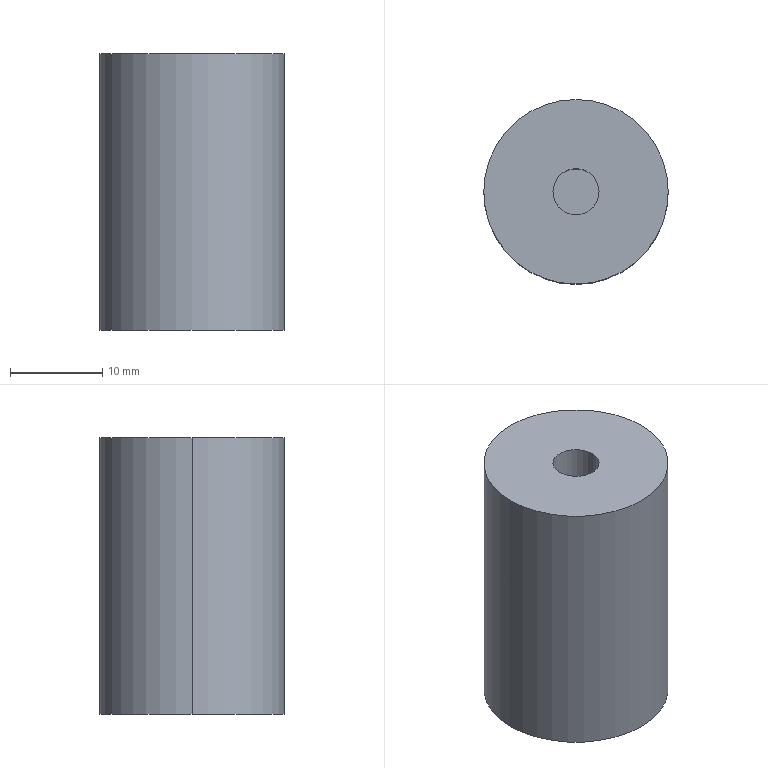Part | SolidWorks | features BaseBody 1 | 1 solid | 10 faces | box 20 x 20 x 30 mm | volume 8586 mm3 | cylinder 6 | plane 4 | commonest cylinder face diameters 5 x2 8 x2 20 x2
STEP:
#1=CARTESIAN_POINT('',(-10.,0.,30.));
#2=VERTEX_POINT('',#1);
#3=CARTESIAN_POINT('',(10.,0.,30.));
#4=VERTEX_POINT('',#3);
#5=CARTESIAN_POINT('',(0.,0.,30.));
#6=DIRECTION('',(0.,0.,-1.));
#7=DIRECTION('',(-1.,0.,0.));
#8=AXIS2_PLACEMENT_3D('',#5,#6,#7);
#9=CIRCLE('',#8,10.);
#10=EDGE_CURVE('',#2,#4,#9,.T.);
#11=ORIENTED_EDGE('',*,*,#10,.T.);
#12=CARTESIAN_POINT('',(10.,0.,0.));
#13=VERTEX_POINT('',#12);
#14=CARTESIAN_POINT('',(10.,0.,30.));
#15=DIRECTION('',(0.,0.,-1.));
#16=VECTOR('',#15,1000.);
#17=LINE('',#14,#16);
#18=EDGE_CURVE('',#4,#13,#17,.T.);
#19=ORIENTED_EDGE('',*,*,#18,.T.);
#20=CARTESIAN_POINT('',(-10.,0.,0.));
#21=VERTEX_POINT('',#20);
#22=CARTESIAN_POINT('',(0.,0.,0.));
#23=DIRECTION('',(0.,0.,1.));
#24=DIRECTION('',(-1.,0.,0.));
#25=AXIS2_PLACEMENT_3D('',#22,#23,#24);
#26=CIRCLE('',#25,10.);
#27=EDGE_CURVE('',#13,#21,#26,.T.);
#28=ORIENTED_EDGE('',*,*,#27,.T.);
#29=CARTESIAN_POINT('',(-10.,0.,30.));
#30=DIRECTION('',(0.,0.,-1.));
#31=VECTOR('',#30,1000.);
#32=LINE('',#29,#31);
#33=EDGE_CURVE('',#2,#21,#32,.T.);
#34=ORIENTED_EDGE('',*,*,#33,.F.);
#35=EDGE_LOOP('',(#11,#19,#28,#34));
#36=FACE_OUTER_BOUND('',#35,.T.);
#37=CARTESIAN_POINT('',(0.,0.,30.));
#38=DIRECTION('',(0.,0.,-1.));
#39=DIRECTION('',(-1.,0.,0.));
#40=AXIS2_PLACEMENT_3D('',#37,#38,#39);
#41=CYLINDRICAL_SURFACE('',#40,10.);
#42=ADVANCED_FACE('',(#36),#41,.T.);
#43=CARTESIAN_POINT('',(4.,0.,12.));
#44=VERTEX_POINT('',#43);
#45=CARTESIAN_POINT('',(-4.,0.,12.));
#46=VERTEX_POINT('',#45);
#47=CARTESIAN_POINT('',(0.,0.,12.));
#48=DIRECTION('',(0.,0.,-1.));
#49=DIRECTION('',(-1.,0.,0.));
#50=AXIS2_PLACEMENT_3D('',#47,#48,#49);
#51=CIRCLE('',#50,4.);
#52=EDGE_CURVE('',#44,#46,#51,.T.);
#53=ORIENTED_EDGE('',*,*,#52,.F.);
#54=CARTESIAN_POINT('',(4.,0.,0.));
#55=VERTEX_POINT('',#54);
#56=CARTESIAN_POINT('',(4.,0.,12.));
#57=DIRECTION('',(0.,0.,-1.));
#58=VECTOR('',#57,1000.);
#59=LINE('',#56,#58);
#60=EDGE_CURVE('',#44,#55,#59,.T.);
#61=ORIENTED_EDGE('',*,*,#60,.T.);
#62=CARTESIAN_POINT('',(-4.,0.,0.));
#63=VERTEX_POINT('',#62);
#64=CARTESIAN_POINT('',(0.,0.,0.));
#65=DIRECTION('',(0.,0.,-1.));
#66=DIRECTION('',(-1.,0.,0.));
#67=AXIS2_PLACEMENT_3D('',#64,#65,#66);
#68=CIRCLE('',#67,4.);
#69=EDGE_CURVE('',#55,#63,#68,.T.);
#70=ORIENTED_EDGE('',*,*,#69,.T.);
#71=CARTESIAN_POINT('',(-4.,0.,12.));
#72=DIRECTION('',(0.,0.,-1.));
#73=VECTOR('',#72,1000.);
#74=LINE('',#71,#73);
#75=EDGE_CURVE('',#46,#63,#74,.T.);
#76=ORIENTED_EDGE('',*,*,#75,.F.);
#77=EDGE_LOOP('',(#53,#61,#70,#76));
#78=FACE_OUTER_BOUND('',#77,.T.);
#79=CARTESIAN_POINT('',(0.,0.,12.));
#80=DIRECTION('',(0.,0.,-1.));
#81=DIRECTION('',(-1.,0.,0.));
#82=AXIS2_PLACEMENT_3D('',#79,#80,#81);
#83=CYLINDRICAL_SURFACE('',#82,4.);
#84=ADVANCED_FACE('',(#78),#83,.F.);
#85=CARTESIAN_POINT('',(-2.5,0.,18.));
#86=VERTEX_POINT('',#85);
#87=CARTESIAN_POINT('',(2.5,0.,18.));
#88=VERTEX_POINT('',#87);
#89=CARTESIAN_POINT('',(0.,0.,18.));
#90=DIRECTION('',(0.,0.,1.));
#91=DIRECTION('',(1.,0.,0.));
#92=AXIS2_PLACEMENT_3D('',#89,#90,#91);
#93=CIRCLE('',#92,2.5);
#94=EDGE_CURVE('',#86,#88,#93,.T.);
#95=ORIENTED_EDGE('',*,*,#94,.F.);
#96=CARTESIAN_POINT('',(-2.5,0.,30.));
#97=VERTEX_POINT('',#96);
#98=CARTESIAN_POINT('',(-2.5,0.,18.));
#99=DIRECTION('',(0.,0.,1.));
#100=VECTOR('',#99,1000.);
#101=LINE('',#98,#100);
#102=EDGE_CURVE('',#86,#97,#101,.T.);
#103=ORIENTED_EDGE('',*,*,#102,.T.);
#104=CARTESIAN_POINT('',(2.5,0.,30.));
#105=VERTEX_POINT('',#104);
#106=CARTESIAN_POINT('',(0.,0.,30.));
#107=DIRECTION('',(0.,0.,-1.));
#108=DIRECTION('',(1.,0.,0.));
#109=AXIS2_PLACEMENT_3D('',#106,#107,#108);
#110=CIRCLE('',#109,2.5);
#111=EDGE_CURVE('',#105,#97,#110,.T.);
#112=ORIENTED_EDGE('',*,*,#111,.F.);
#113=CARTESIAN_POINT('',(2.5,0.,18.));
#114=DIRECTION('',(0.,0.,1.));
#115=VECTOR('',#114,1000.);
#116=LINE('',#113,#115);
#117=EDGE_CURVE('',#88,#105,#116,.T.);
#118=ORIENTED_EDGE('',*,*,#117,.F.);
#119=EDGE_LOOP('',(#95,#103,#112,#118));
#120=FACE_OUTER_BOUND('',#119,.T.);
#121=CARTESIAN_POINT('',(0.,0.,18.));
#122=DIRECTION('',(0.,0.,1.));
#123=DIRECTION('',(1.,0.,0.));
#124=AXIS2_PLACEMENT_3D('',#121,#122,#123);
#125=CYLINDRICAL_SURFACE('',#124,2.5);
#126=ADVANCED_FACE('',(#120),#125,.F.);
#127=ORIENTED_EDGE('',*,*,#18,.F.);
#128=CARTESIAN_POINT('',(0.,0.,30.));
#129=DIRECTION('',(0.,0.,-1.));
#130=DIRECTION('',(-1.,0.,0.));
#131=AXIS2_PLACEMENT_3D('',#128,#129,#130);
#132=CIRCLE('',#131,10.);
#133=EDGE_CURVE('',#4,#2,#132,.T.);
#134=ORIENTED_EDGE('',*,*,#133,.T.);
#135=ORIENTED_EDGE('',*,*,#33,.T.);
#136=CARTESIAN_POINT('',(0.,0.,0.));
#137=DIRECTION('',(0.,0.,1.));
#138=DIRECTION('',(-1.,0.,0.));
#139=AXIS2_PLACEMENT_3D('',#136,#137,#138);
#140=CIRCLE('',#139,10.);
#141=EDGE_CURVE('',#21,#13,#140,.T.);
#142=ORIENTED_EDGE('',*,*,#141,.T.);
#143=EDGE_LOOP('',(#127,#134,#135,#142));
#144=FACE_OUTER_BOUND('',#143,.T.);
#145=CARTESIAN_POINT('',(0.,0.,30.));
#146=DIRECTION('',(0.,0.,-1.));
#147=DIRECTION('',(-1.,0.,0.));
#148=AXIS2_PLACEMENT_3D('',#145,#146,#147);
#149=CYLINDRICAL_SURFACE('',#148,10.);
#150=ADVANCED_FACE('',(#144),#149,.T.);
#151=ORIENTED_EDGE('',*,*,#141,.F.);
#152=ORIENTED_EDGE('',*,*,#27,.F.);
#153=EDGE_LOOP('',(#151,#152));
#154=FACE_OUTER_BOUND('',#153,.T.);
#155=CARTESIAN_POINT('',(0.,0.,0.));
#156=DIRECTION('',(0.,0.,-1.));
#157=DIRECTION('',(-1.,0.,0.));
#158=AXIS2_PLACEMENT_3D('',#155,#156,#157);
#159=CIRCLE('',#158,4.);
#160=EDGE_CURVE('',#63,#55,#159,.T.);
#161=ORIENTED_EDGE('',*,*,#160,.F.);
#162=ORIENTED_EDGE('',*,*,#69,.F.);
#163=EDGE_LOOP('',(#161,#162));
#164=FACE_BOUND('',#163,.T.);
#165=CARTESIAN_POINT('',(0.,0.,0.));
#166=DIRECTION('',(0.,0.,1.));
#167=DIRECTION('',(1.,0.,0.));
#168=AXIS2_PLACEMENT_3D('',#165,#166,#167);
#169=PLANE('',#168);
#170=ADVANCED_FACE('',(#154,#164),#169,.F.);
#171=ORIENTED_EDGE('',*,*,#10,.F.);
#172=ORIENTED_EDGE('',*,*,#133,.F.);
#173=EDGE_LOOP('',(#171,#172));
#174=FACE_OUTER_BOUND('',#173,.T.);
#175=ORIENTED_EDGE('',*,*,#111,.T.);
#176=CARTESIAN_POINT('',(0.,0.,30.));
#177=DIRECTION('',(0.,0.,-1.));
#178=DIRECTION('',(1.,0.,0.));
#179=AXIS2_PLACEMENT_3D('',#176,#177,#178);
#180=CIRCLE('',#179,2.5);
#181=EDGE_CURVE('',#97,#105,#180,.T.);
#182=ORIENTED_EDGE('',*,*,#181,.T.);
#183=EDGE_LOOP('',(#175,#182));
#184=FACE_BOUND('',#183,.T.);
#185=CARTESIAN_POINT('',(0.,0.,30.));
#186=DIRECTION('',(0.,0.,1.));
#187=DIRECTION('',(1.,0.,0.));
#188=AXIS2_PLACEMENT_3D('',#185,#186,#187);
#189=PLANE('',#188);
#190=ADVANCED_FACE('',(#174,#184),#189,.T.);
#191=ORIENTED_EDGE('',*,*,#60,.F.);
#192=CARTESIAN_POINT('',(0.,0.,12.));
#193=DIRECTION('',(0.,0.,-1.));
#194=DIRECTION('',(-1.,0.,0.));
#195=AXIS2_PLACEMENT_3D('',#192,#193,#194);
#196=CIRCLE('',#195,4.);
#197=EDGE_CURVE('',#46,#44,#196,.T.);
#198=ORIENTED_EDGE('',*,*,#197,.F.);
#199=ORIENTED_EDGE('',*,*,#75,.T.);
#200=ORIENTED_EDGE('',*,*,#160,.T.);
#201=EDGE_LOOP('',(#191,#198,#199,#200));
#202=FACE_OUTER_BOUND('',#201,.T.);
#203=CARTESIAN_POINT('',(0.,0.,12.));
#204=DIRECTION('',(0.,0.,-1.));
#205=DIRECTION('',(-1.,0.,0.));
#206=AXIS2_PLACEMENT_3D('',#203,#204,#205);
#207=CYLINDRICAL_SURFACE('',#206,4.);
#208=ADVANCED_FACE('',(#202),#207,.F.);
#209=ORIENTED_EDGE('',*,*,#102,.F.);
#210=CARTESIAN_POINT('',(0.,0.,18.));
#211=DIRECTION('',(0.,0.,1.));
#212=DIRECTION('',(1.,0.,0.));
#213=AXIS2_PLACEMENT_3D('',#210,#211,#212);
#214=CIRCLE('',#213,2.5);
#215=EDGE_CURVE('',#88,#86,#214,.T.);
#216=ORIENTED_EDGE('',*,*,#215,.F.);
#217=ORIENTED_EDGE('',*,*,#117,.T.);
#218=ORIENTED_EDGE('',*,*,#181,.F.);
#219=EDGE_LOOP('',(#209,#216,#217,#218));
#220=FACE_OUTER_BOUND('',#219,.T.);
#221=CARTESIAN_POINT('',(0.,0.,18.));
#222=DIRECTION('',(0.,0.,1.));
#223=DIRECTION('',(1.,0.,0.));
#224=AXIS2_PLACEMENT_3D('',#221,#222,#223);
#225=CYLINDRICAL_SURFACE('',#224,2.5);
#226=ADVANCED_FACE('',(#220),#225,.F.);
#227=ORIENTED_EDGE('',*,*,#197,.T.);
#228=ORIENTED_EDGE('',*,*,#52,.T.);
#229=EDGE_LOOP('',(#227,#228));
#230=FACE_OUTER_BOUND('',#229,.T.);
#231=CARTESIAN_POINT('',(0.,0.,12.));
#232=DIRECTION('',(0.,0.,-1.));
#233=DIRECTION('',(-1.,0.,0.));
#234=AXIS2_PLACEMENT_3D('',#231,#232,#233);
#235=PLANE('',#234);
#236=ADVANCED_FACE('',(#230),#235,.T.);
#237=ORIENTED_EDGE('',*,*,#215,.T.);
#238=ORIENTED_EDGE('',*,*,#94,.T.);
#239=EDGE_LOOP('',(#237,#238));
#240=FACE_OUTER_BOUND('',#239,.T.);
#241=CARTESIAN_POINT('',(0.,0.,18.));
#242=DIRECTION('',(0.,0.,1.));
#243=DIRECTION('',(1.,0.,0.));
#244=AXIS2_PLACEMENT_3D('',#241,#242,#243);
#245=PLANE('',#244);
#246=ADVANCED_FACE('',(#240),#245,.T.);
#247=CLOSED_SHELL('',(#42,#84,#126,#150,#170,#190,#208,#226,#236,#246));
#248=MANIFOLD_SOLID_BREP('',#247);
#249=CARTESIAN_POINT('',(0.,0.,0.));
#250=DIRECTION('',(0.,0.,1.));
#251=DIRECTION('',(1.,0.,0.));
#252=AXIS2_PLACEMENT_3D('',#249,#250,#251);
#253=(LENGTH_UNIT()NAMED_UNIT(*)SI_UNIT(.MILLI.,.METRE.));
#254=UNCERTAINTY_MEASURE_WITH_UNIT(LENGTH_MEASURE(0.00001),#253,'','');
#255=(NAMED_UNIT(*)PLANE_ANGLE_UNIT()SI_UNIT($,.RADIAN.));
#256=(NAMED_UNIT(*)SI_UNIT($,.STERADIAN.)SOLID_ANGLE_UNIT());
#257=(GEOMETRIC_REPRESENTATION_CONTEXT(3)GLOBAL_UNCERTAINTY_ASSIGNED_CONTEXT((#254))GLOBAL_UNIT_ASSIGNED_CONTEXT((#253,#255,#256))REPRESENTATION_CONTEXT('',''));
#258=ADVANCED_BREP_SHAPE_REPRESENTATION('',(#248,#252),#257);